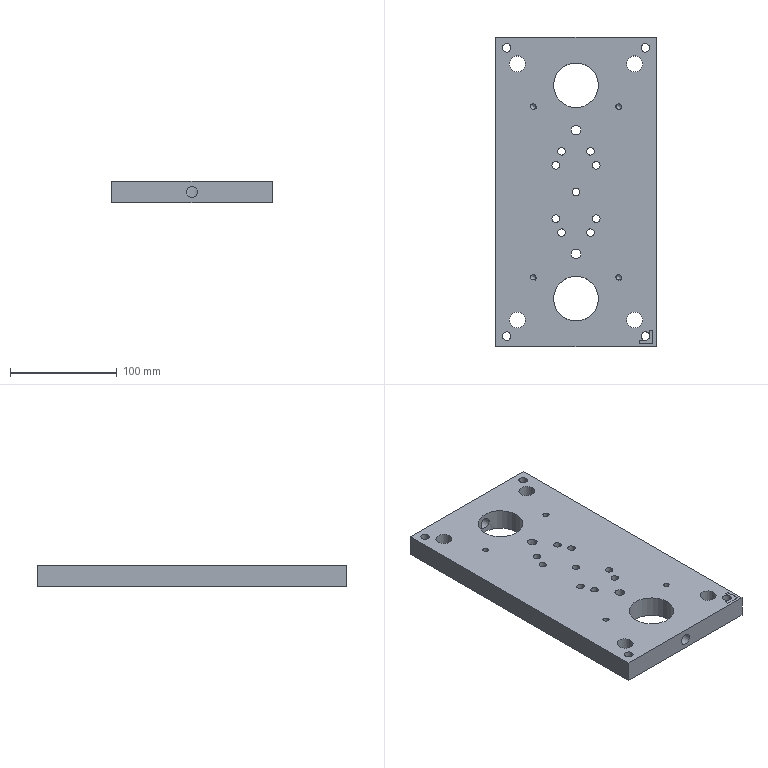Part | STEP file | DZMB_id258_x_t | 1 solid | 82 faces | box 150 x 290 x 20 mm | volume 774159 mm3 | cylinder 50 | plane 28 | cone 4 | commonest cylinder face diameters 7 x9 11 x9 6 x8 5 x4 8 x4 15 x4